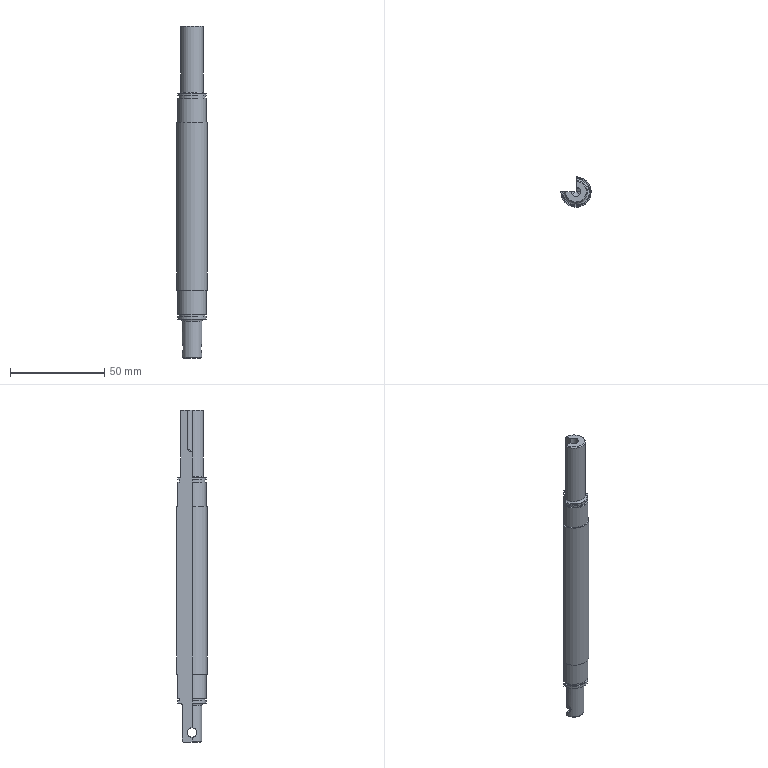Part | STEP file | drive shaft | 1 solid | 35 faces | box 16 x 16 x 176 mm | volume 21338 mm3 | cylinder 14 | plane 13 | cone 5 | torus 3 | commonest cylinder face diameters 5 x4 15 x4 13.8 x3 10.5 x1 12 x1 16 x1